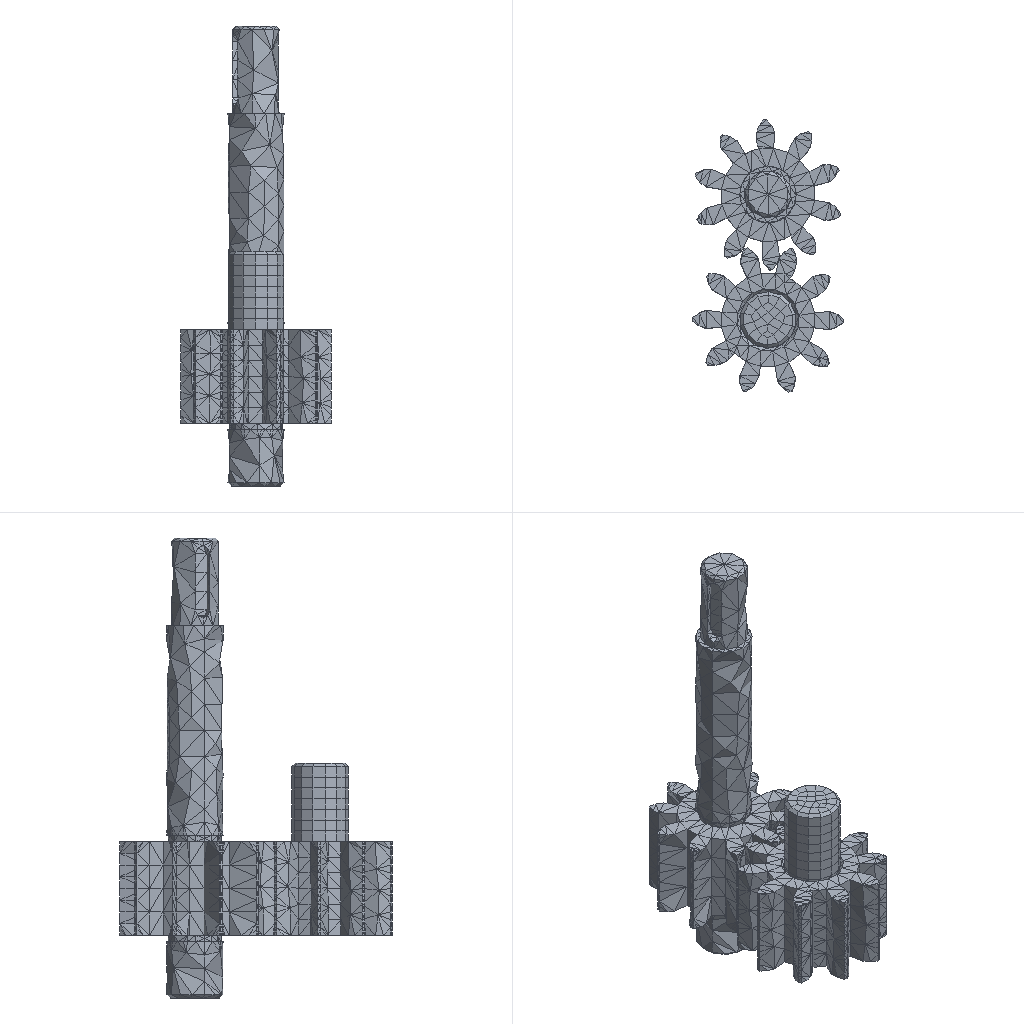Simulation study | ansys workbench
Ansys APDL input file, long lists of numbers shortened:
/batch
/config,noeldb,1     ! force off writing results to database
*get,_wallstrt,active,,time,wall
! ANSYS input file written by Workbench version 2022 R1
! File used for geometry attach:
/title,wbnew--____ (B5)
! ****** Begin Custom Load Command Snippet ******
/COM, ACT Extensions:
/COM,     LSDYNA, 2021.1
/COM,
! ****** End   Custom Load Command Snippet ******
*DIM,_wb_ProjectScratch_dir,string,248
_wb_ProjectScratch_dir(1) = ''
*DIM,_wb_SolverFiles_dir,string,248
_wb_SolverFiles_dir(1) = ''
*DIM,_wb_userfiles_dir,string,248
_wb_userfiles_dir(1) = ''
/com,--- Data in consistent NMM units. See Solving Units in the help system for more information.
/units,MPA
/nopr
/wb,file,start              !  signify a WB generated input file
/prep7
! Turn off shape checking because checks already performed inside WB mesher.
! See help system for more information.
SHPP,OFF,,NOWARN
/nolist
etcon,set             ! allow ANSYS to choose best KEYOP's for 180x elements, resets any applicable keyopt to MAPDL defaults
/com,*********** Nodes for the whole assembly ***********
nblock,3,,14512
(1i9,3e20.9e3)
        1    -2.338007419E+01    -1.072781647E+01     1.600000000E+01
! (13192 more lines like these left out)
-1
/com,*********** Nodes for all Remote Points ***********
nblock,3
(1i9,3e20.9e3)
    13194    -1.762855123E+01     1.925884634E+01     7.534549748E+00
-1
/wb,elem,start            !  set before creation of elements
/com,*********** Elements for Body 1 "___GB - Spur gear 4M 10T 20PA 30FW ---S10A75H55L18.0N|NONE" ***********
et,1,187
eblock,19,solid,,2531
(19i9)
        1        1        1        1        0        0        0        0       10        0      444     3020     3121     3228     3210     6903     7297     6907     6906
! (5061 more lines like these left out)
-1
/com,*********** Elements for Body 2 "___|NONE" ***********
et,2,186
keyo,2,2,1          ! set full integration on SOLID186
eblock,19,solid,,243
(19i9)
        2        2        2        2        0        0        0        0       20        0      201     1075     1076     1083     1093     1263     1262     1255     1245
! (485 more lines like these left out)
-1
/com,*********** Elements for Body 3 "___|NONE[2]" ***********
et,3,186
keyo,3,2,1          ! set full integration on SOLID186
eblock,19,solid,,200
(19i9)
        3        3        3        3        0        0        0        0       20        0        1        1        2       12        4      152      151      141      149
! (399 more lines like these left out)
-1
/com,*********** Elements for Body 4 "___GB - Spur gear 4M 10T 20PA 30FW ---S10A75H55L10.0N|NONE" ***********
et,4,187
eblock,19,solid,,2942
(19i9)
        4        4        4        4        0        0        0        0       10        0     2975     8337     8385     8419     8386    13031    13179    13037    13032
! (5883 more lines like these left out)
-1
/wb,elem,end               !  done creating elements
/com,*********** Send User Defined Coordinate System(s) ***********
csys,0
toffst,273.15,  ! Temperature offset from absolute zero
/com,*********** Set Reference Temperature ***********
tref,22.
/wb,mat,start              !  starting to send materials
/com,*********** Send Materials ***********
Temperature = 'TEMP' ! Temperature
MP,DENS,1,7.85e-09,	! tonne mm^-3
MP,ALPX,1,1.2e-05,	! C^-1
MP,C,1,434000000,	! mm^2 s^-2 C^-1
MP,KXX,1,60.5,	! tonne mm s^-3 C^-1
MP,RSVX,1,0.00017,	! ohm mm
MP,EX,1,200000,	! tonne s^-2 mm^-1
MP,NUXY,1,0.3,
MP,MURX,1,10000,
Temperature = 'TEMP' ! Temperature
MP,DENS,2,7.85e-09,	! tonne mm^-3
MP,ALPX,2,1.2e-05,	! C^-1
MP,C,2,434000000,	! mm^2 s^-2 C^-1
MP,KXX,2,60.5,	! tonne mm s^-3 C^-1
MP,RSVX,2,0.00017,	! ohm mm
MP,EX,2,200000,	! tonne s^-2 mm^-1
MP,NUXY,2,0.3,
MP,MURX,2,10000,
Temperature = 'TEMP' ! Temperature
MP,DENS,3,7.85e-09,	! tonne mm^-3
MP,ALPX,3,1.2e-05,	! C^-1
MP,C,3,434000000,	! mm^2 s^-2 C^-1
MP,KXX,3,60.5,	! tonne mm s^-3 C^-1
MP,RSVX,3,0.00017,	! ohm mm
MP,EX,3,200000,	! tonne s^-2 mm^-1
MP,NUXY,3,0.3,
MP,MURX,3,10000,
Temperature = 'TEMP' ! Temperature
MP,DENS,4,7.85e-09,	! tonne mm^-3
MP,ALPX,4,1.2e-05,	! C^-1
MP,C,4,434000000,	! mm^2 s^-2 C^-1
MP,KXX,4,60.5,	! tonne mm s^-3 C^-1
MP,RSVX,4,0.00017,	! ohm mm
MP,EX,4,200000,	! tonne s^-2 mm^-1
MP,NUXY,4,0.3,
MP,MURX,4,10000,
/wb,mat,end                !  done sending materials
!************************* Model Summary ********************
!___GB - Spur gear 4M 10T 20PA 30FW ---S10A75H55L18.0N|NONE,	结构钢,	matid,	1
!___|NONE,	结构钢,	matid,	2
!___|NONE[2],	结构钢,	matid,	3
!___GB - Spur gear 4M 10T 20PA 30FW ---S10A75H55L10.0N|NONE,	结构钢,	matid,	4
!************************* End Model Summary ********************
! get the diagonal of the bounding box. Needed later for other things
*get,_xmin,node,,mnloc,x
*get,_ymin,node,,mnloc,y
*get,_zmin,node,,mnloc,z
*get,_xmax,node,,mxloc,x
*get,_ymax,node,,mxloc,y
*get,_zmax,node,,mxloc,z
_ASMDIAG=(_xmax-_xmin)*(_xmax-_xmin)+(_ymax-_ymin)*(_ymax-_ymin)+(_zmax-_zmin)*(_zmax-_zmin)
_ASMDIAG=SQRT(_ASMDIAG)
/wb,contact,start          !  starting to send contact
/com,*********** Create Contact "接触区域" ***********
/com,            Real Constant Set For Above Contact Is 6 & 5
*set,tid,6
*set,cid,5
r,tid
r,cid
et,tid,170
et,cid,174
eblock,10,,,160
(15i9)
     9438        6        6        6        0     2793     2381     2382     2382     3423     3418     2382     3430
! (159 more lines like these left out)
-1
eblock,10,,,160
(15i9)
     9598        5        5        5        0     2793     2381     2382     2382     3423     3418     2382     3430
! (159 more lines like these left out)
-1
eblock,10,,,112
(15i9)
     9758        5        6        5        0     1363     1315     1314     1307     2148     2145     2129     2130
! (111 more lines like these left out)
-1
eblock,10,,,112
(15i9)
     9870        6        5        6        0     1363     1315     1314     1307     2148     2145     2129     2130
! (111 more lines like these left out)
-1
keyo,cid,8,2               ! auto create asymmetric contact (from Program Controlled setting)
keyo,cid,10,0              ! adjust contact stiffness each NR iteration (from Program Controlled setting)
keyo,cid,12,5              ! bonded always
keyo,cid,18,1              ! small sliding turned on by application
keyo,cid,2,0               ! augmented Lagrange (from Program Controlled setting)
keyo,cid,4,0               ! on Gauss point (from Program Controlled setting)
keyo,cid,9,1               ! ignore initial gaps/penetration
keyo,cid,7,0               ! No Prediction
rmod,tid,3,10.      ! FKN
rmod,tid,5,0.       ! ICONT
rmod,tid,6,0.       ! PINB
rmod,tid,10,0.      ! CNOF
rmod,tid,12,0.      ! FKT
rmod,tid,36,35      ! WB DSID
rmod,cid,3,10.      ! FKN
rmod,cid,5,0.       ! ICONT
rmod,cid,6,0.       ! PINB
rmod,cid,10,0.      ! CNOF
rmod,cid,12,0.      ! FKT
rmod,cid,36,35      ! WB DSID
/com,*********** Create Contact "接触区域 2" ***********
/com,            Real Constant Set For Above Contact Is 8 & 7
*set,tid,8
*set,cid,7
r,tid
r,cid
et,tid,170
et,cid,174
eblock,10,,,26
(15i9)
     9982        8        8        8        0     2530     2858     2859     2859     4522     6421     2859     4523
! (25 more lines like these left out)
-1
eblock,10,,,26
(15i9)
    10008        7        7        7        0     2530     2858     2859     2859     4522     6421     2859     4523
! (25 more lines like these left out)
-1
eblock,10,,,18
(15i9)
    10034        7        8        7        0     7772     8049     8055     8055    10911    11961     8055    10912
! (17 more lines like these left out)
-1
eblock,10,,,18
(15i9)
    10052        8        7        8        0     7772     8049     8055     8055    10911    11961     8055    10912
! (17 more lines like these left out)
-1
keyo,cid,8,2               ! auto create asymmetric contact (from Program Controlled setting)
keyo,cid,10,0              ! adjust contact stiffness each NR iteration (from Program Controlled setting)
keyo,cid,12,5              ! bonded always
keyo,cid,18,1              ! small sliding turned on by application
keyo,cid,2,0               ! augmented Lagrange (from Program Controlled setting)
keyo,cid,4,0               ! on Gauss point (from Program Controlled setting)
keyo,cid,9,1               ! ignore initial gaps/penetration
keyo,cid,7,0               ! No Prediction
rmod,tid,3,10.      ! FKN
rmod,tid,5,0.       ! ICONT
rmod,tid,6,0.       ! PINB
rmod,tid,10,0.      ! CNOF
rmod,tid,12,0.      ! FKT
rmod,tid,36,38      ! WB DSID
rmod,cid,3,10.      ! FKN
rmod,cid,5,0.       ! ICONT
rmod,cid,6,0.       ! PINB
rmod,cid,10,0.      ! CNOF
rmod,cid,12,0.      ! FKT
rmod,cid,36,38      ! WB DSID
/com,*********** Create Contact "接触区域 3" ***********
/com,            Real Constant Set For Above Contact Is 10 & 9
*set,tid,10
*set,cid,9
r,tid
r,cid
et,tid,170
et,cid,174
eblock,10,,,27
(15i9)
    10070       10       10       10        0     1282     1272     1265     1264     2064     2041     2037     2039
! (26 more lines like these left out)
-1
eblock,10,,,27
(15i9)
    10097        9        9        9        0     1282     1272     1265     1264     2064     2041     2037     2039
! (26 more lines like these left out)
-1
eblock,10,,,25
(15i9)
    10124        9       10        9        0      156      164      154      153      806      800      794      795
! (24 more lines like these left out)
-1
eblock,10,,,25
(15i9)
    10149       10        9       10        0      156      164      154      153      806      800      794      795
! (24 more lines like these left out)
-1
keyo,cid,8,2               ! auto create asymmetric contact (from Program Controlled setting)
keyo,cid,10,0              ! adjust contact stiffness each NR iteration (from Program Controlled setting)
keyo,cid,12,5              ! bonded always
keyo,cid,18,1              ! small sliding turned on by application
keyo,cid,2,0               ! augmented Lagrange (from Program Controlled setting)
keyo,cid,4,0               ! on Gauss point (from Program Controlled setting)
keyo,cid,9,1               ! ignore initial gaps/penetration
keyo,cid,7,0               ! No Prediction
rmod,tid,3,10.      ! FKN
rmod,tid,5,0.       ! ICONT
rmod,tid,6,0.       ! PINB
rmod,tid,10,0.      ! CNOF
rmod,tid,12,0.      ! FKT
rmod,tid,36,41      ! WB DSID
rmod,cid,3,10.      ! FKN
rmod,cid,5,0.       ! ICONT
rmod,cid,6,0.       ! PINB
rmod,cid,10,0.      ! CNOF
rmod,cid,12,0.      ! FKT
rmod,cid,36,41      ! WB DSID
nsel,all
esel,all
/wb,contact,end            !  done creating contacts
/golist
/wb,load,start             !  starting to send loads
CMBLOCK,_CM49_FIXEDSU,NODE,      693
(8i10)
       172       173       174       175       176       177       178       179
! (86 more lines like these left out)
/com,*********** Fixed Supports ***********
CMBLOCK,_FIXEDSU,NODE,      693
(8i10)
       172       173       174       175       176       177       178       179
! (86 more lines like these left out)
cmsel,s,_FIXEDSU
d,all,all
nsel,all
/com,*********** Create Remote Point "内部远程点" ***********
! -------- Remote Point Used by "力矩" --------
*set,tid,12
*set,cid,11
et,cid,174
et,tid,170
keyo,tid,2,1               ! Don't fix the pilot node
keyo,tid,4,111111
keyo,cid,12,5              ! Bonded Contact
keyo,cid,4,1               ! Deformable RBE3 style load
keyo,cid,2,2               ! MPC style contact
eblock,10,,,416
(15i9)
    10174       11       11       11        0     7557     7895     7901     7901     9476    11528     7901     9477
! (415 more lines like these left out)
-1
*set,_npilot,13194
_npilot52=_npilot
type,tid
mat ,cid
real,cid
tshape,pilo
en,10590,_npilot
tshape
/com,*********** Construct Moment Using Remote Attachment ***********
/gst,on,on
fini
*get,_numnode,node,0,count
*get,_numelem,elem,0,count
*get, _MAXELEMNUM, elem, 0, NUM, MAX
*get, _MAXNODENUM, node, 0, NUM, MAX
*get, _MAXELEMTYPE, etyp, 0, NUM, MAX
*get, _MAXREALCONST, real, 0, NUM, MAX
/go
/wb,load,end               !  done creating loads
/com,--- Number of total nodes = %_numnode%
/com,--- Number of contact elements = 1152
/com,--- Number of spring elements = 0
/com,--- Number of bearing elements = 0
/com,--- Number of solid elements = 5916
/com,--- Number of condensed parts = 0
/com,--- Number of total elements = %_numelem%
*get,_wallbsol,active,,time,wall
/com,****************************************************************************
/com,*************************    SOLUTION       ********************************
/com,****************************************************************************
/solu
antype,0                   ! static analysis
_thickRatio=0.75    ! Ratio of thick parts in the model
eqsl,pcg,1e-8,,,,,,1
cntr,print,1               ! print out contact info and also make no initial contact an error
nldiag,cont,iter           ! print out contact info each equilibrium iteration
rescontrol,linear,last           ! Turn on restart files due to future eigen analysis intent
/com,****************************************************
/com,******************* SOLVE FOR LS 1 OF 1 ****************
nsel,s,node,,13194
f,all,mx,0.
f,all,my,0.
f,all,mz,50000.
nsel,all
/nopr
/gopr
nsub,1,1,1
time,1.
outres,erase
outres,all,none
outres,nsol,all,
outres,rsol,all
outres,eangl,all
outres,etmp,all
outres,veng,all
outres,strs,all,
outres,epel,all,
outres,eppl,all,
outres,cont,all,
! *********** WB SOLVE COMMAND ***********
! check interactive state
*get,ANSINTER_,active,,int
*if,ANSINTER_,ne,0,then
/eof
*endif
solve
/com *************** Write FE CONNECTORS *********
CEWRITE,file,ce,,INTE
/com,****************************************************
/com,*************** FINISHED SOLVE FOR LS 1 *************
*get,_wallasol,active,,time,wall
/nopr
*get,_numnode,node,0,count
*get,_numelem,elem,0,count
*get, _MAXELEMNUM, elem, 0, NUM, MAX
*get, _MAXNODENUM, node, 0, NUM, MAX,,,INTERNAL
*get, _MAXELEMTYPE, etyp, 0, NUM, MAX
*get, _MAXREALCONST, real, 0, NUM, MAX
/gopr
*get,_PCGITER,active,,solu,cgiter
/post1
xmlo,ENCODING,ISO-8859-1
xmlo,parm
/xml,parm,xml
fini
/gopr
*get,_walldone,active,,time,wall
_preptime=(_wallbsol-_wallstrt)*3600
_solvtime=(_wallasol-_wallbsol)*3600
_posttime=(_walldone-_wallasol)*3600
_totaltim=(_walldone-_wallstrt)*3600
*get,_dlbratio,active,0,solu,dlbr
*get,_combtime,active,0,solu,comb
*get,_ssmode,active,0,solu,ssmm
*get,_ndofs,active,0,solu,ndof
/com,--- Total number of nodes = %_numnode%
/com,--- Total number of elements = %_numelem%
/com,--- Element load balance ratio = %_dlbratio%
/com,--- Time to combine distributed files = %_combtime%
/com,--- Sparse memory mode = %_ssmode%
/com,--- Number of DOF = %_ndofs%
/wb,file,end               ! done with WB generated input